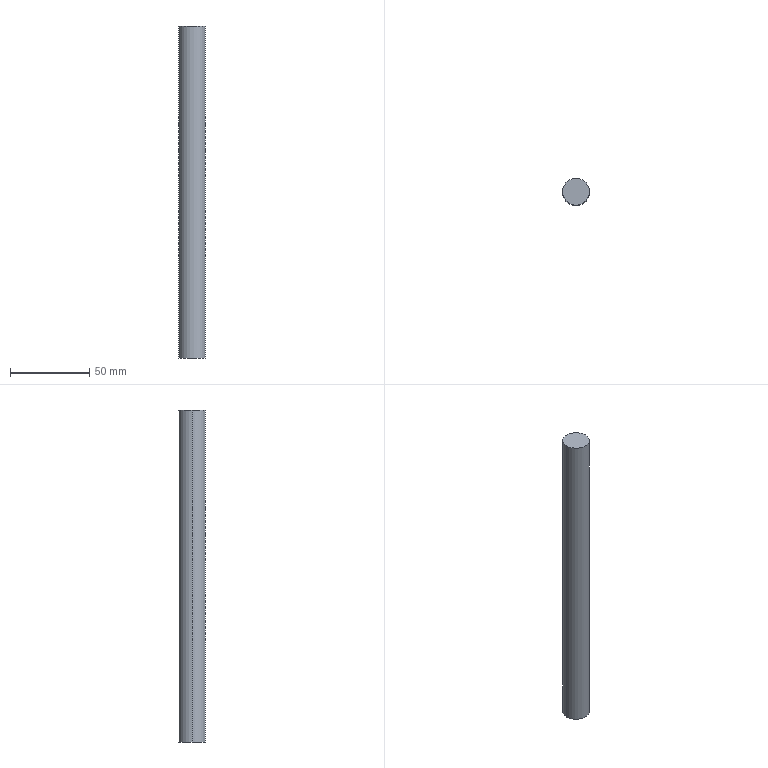Part | SolidWorks | features Extrusion 1 | 1 solid | 4 faces | box 17 x 17 x 210 mm | volume 47666 mm3 | cylinder 2 | plane 2 | commonest cylinder face diameters 17 x2
STEP:
#1=CARTESIAN_POINT('',(8.5,0.,210.));
#2=VERTEX_POINT('',#1);
#3=CARTESIAN_POINT('',(-8.5,0.,210.));
#4=VERTEX_POINT('',#3);
#5=CARTESIAN_POINT('',(0.,0.,210.));
#6=DIRECTION('',(0.,0.,1.));
#7=DIRECTION('',(1.,0.,0.));
#8=AXIS2_PLACEMENT_3D('',#5,#6,#7);
#9=CIRCLE('',#8,8.5);
#10=EDGE_CURVE('',#2,#4,#9,.T.);
#11=ORIENTED_EDGE('',*,*,#10,.F.);
#12=CARTESIAN_POINT('',(8.5,0.,0.));
#13=VERTEX_POINT('',#12);
#14=CARTESIAN_POINT('',(8.5,0.,210.));
#15=DIRECTION('',(0.,0.,-1.));
#16=VECTOR('',#15,1000.);
#17=LINE('',#14,#16);
#18=EDGE_CURVE('',#2,#13,#17,.T.);
#19=ORIENTED_EDGE('',*,*,#18,.T.);
#20=CARTESIAN_POINT('',(-8.5,0.,0.));
#21=VERTEX_POINT('',#20);
#22=CARTESIAN_POINT('',(0.,0.,0.));
#23=DIRECTION('',(0.,0.,1.));
#24=DIRECTION('',(1.,0.,0.));
#25=AXIS2_PLACEMENT_3D('',#22,#23,#24);
#26=CIRCLE('',#25,8.5);
#27=EDGE_CURVE('',#13,#21,#26,.T.);
#28=ORIENTED_EDGE('',*,*,#27,.T.);
#29=CARTESIAN_POINT('',(-8.5,0.,210.));
#30=DIRECTION('',(0.,0.,-1.));
#31=VECTOR('',#30,1000.);
#32=LINE('',#29,#31);
#33=EDGE_CURVE('',#4,#21,#32,.T.);
#34=ORIENTED_EDGE('',*,*,#33,.F.);
#35=EDGE_LOOP('',(#11,#19,#28,#34));
#36=FACE_OUTER_BOUND('',#35,.T.);
#37=CARTESIAN_POINT('',(0.,0.,210.));
#38=DIRECTION('',(0.,0.,-1.));
#39=DIRECTION('',(-1.,0.,0.));
#40=AXIS2_PLACEMENT_3D('',#37,#38,#39);
#41=CYLINDRICAL_SURFACE('',#40,8.5);
#42=ADVANCED_FACE('',(#36),#41,.T.);
#43=ORIENTED_EDGE('',*,*,#18,.F.);
#44=CARTESIAN_POINT('',(0.,0.,210.));
#45=DIRECTION('',(0.,0.,1.));
#46=DIRECTION('',(1.,0.,0.));
#47=AXIS2_PLACEMENT_3D('',#44,#45,#46);
#48=CIRCLE('',#47,8.5);
#49=EDGE_CURVE('',#4,#2,#48,.T.);
#50=ORIENTED_EDGE('',*,*,#49,.F.);
#51=ORIENTED_EDGE('',*,*,#33,.T.);
#52=CARTESIAN_POINT('',(0.,0.,0.));
#53=DIRECTION('',(0.,0.,1.));
#54=DIRECTION('',(1.,0.,0.));
#55=AXIS2_PLACEMENT_3D('',#52,#53,#54);
#56=CIRCLE('',#55,8.5);
#57=EDGE_CURVE('',#21,#13,#56,.T.);
#58=ORIENTED_EDGE('',*,*,#57,.T.);
#59=EDGE_LOOP('',(#43,#50,#51,#58));
#60=FACE_OUTER_BOUND('',#59,.T.);
#61=CARTESIAN_POINT('',(0.,0.,210.));
#62=DIRECTION('',(0.,0.,-1.));
#63=DIRECTION('',(-1.,0.,0.));
#64=AXIS2_PLACEMENT_3D('',#61,#62,#63);
#65=CYLINDRICAL_SURFACE('',#64,8.5);
#66=ADVANCED_FACE('',(#60),#65,.T.);
#67=ORIENTED_EDGE('',*,*,#49,.T.);
#68=ORIENTED_EDGE('',*,*,#10,.T.);
#69=EDGE_LOOP('',(#67,#68));
#70=FACE_OUTER_BOUND('',#69,.T.);
#71=CARTESIAN_POINT('',(0.,0.,210.));
#72=DIRECTION('',(0.,0.,1.));
#73=DIRECTION('',(1.,0.,0.));
#74=AXIS2_PLACEMENT_3D('',#71,#72,#73);
#75=PLANE('',#74);
#76=ADVANCED_FACE('',(#70),#75,.T.);
#77=ORIENTED_EDGE('',*,*,#57,.F.);
#78=ORIENTED_EDGE('',*,*,#27,.F.);
#79=EDGE_LOOP('',(#77,#78));
#80=FACE_OUTER_BOUND('',#79,.T.);
#81=CARTESIAN_POINT('',(0.,0.,0.));
#82=DIRECTION('',(0.,0.,1.));
#83=DIRECTION('',(1.,0.,0.));
#84=AXIS2_PLACEMENT_3D('',#81,#82,#83);
#85=PLANE('',#84);
#86=ADVANCED_FACE('',(#80),#85,.F.);
#87=CLOSED_SHELL('',(#42,#66,#76,#86));
#88=MANIFOLD_SOLID_BREP('',#87);
#89=CARTESIAN_POINT('',(0.,0.,0.));
#90=DIRECTION('',(0.,0.,1.));
#91=DIRECTION('',(1.,0.,0.));
#92=AXIS2_PLACEMENT_3D('',#89,#90,#91);
#93=(LENGTH_UNIT()NAMED_UNIT(*)SI_UNIT(.MILLI.,.METRE.));
#94=UNCERTAINTY_MEASURE_WITH_UNIT(LENGTH_MEASURE(0.00001),#93,'','');
#95=(NAMED_UNIT(*)PLANE_ANGLE_UNIT()SI_UNIT($,.RADIAN.));
#96=(NAMED_UNIT(*)SI_UNIT($,.STERADIAN.)SOLID_ANGLE_UNIT());
#97=(GEOMETRIC_REPRESENTATION_CONTEXT(3)GLOBAL_UNCERTAINTY_ASSIGNED_CONTEXT((#94))GLOBAL_UNIT_ASSIGNED_CONTEXT((#93,#95,#96))REPRESENTATION_CONTEXT('',''));
#98=ADVANCED_BREP_SHAPE_REPRESENTATION('',(#88,#92),#97);